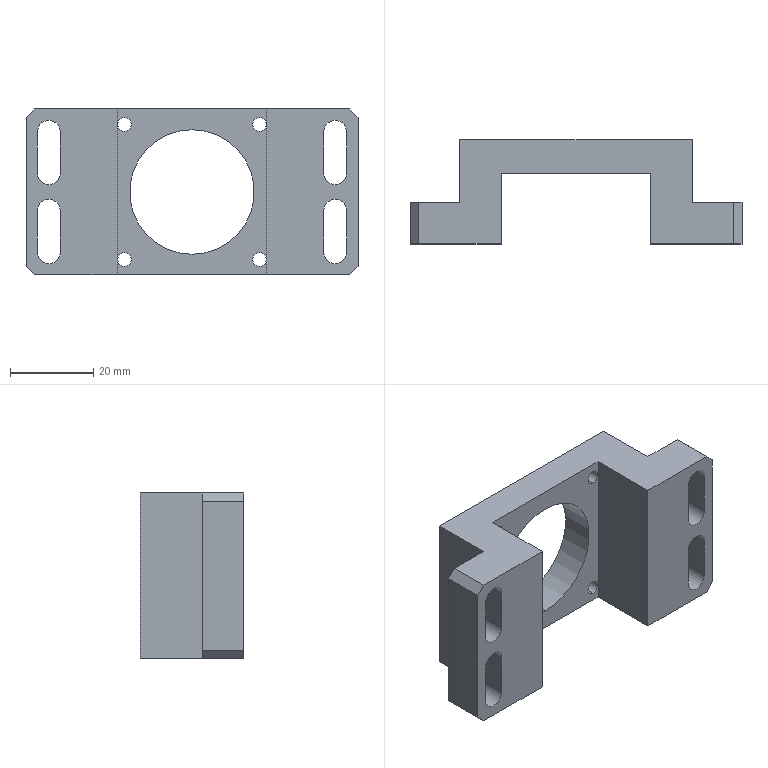Part | STEP file | 06-01-08 motor pad block | 1 solid | 48 faces | box 80 x 25 x 40 mm | volume 31958 mm3 | plane 26 | cylinder 22 | commonest cylinder face diameters 5.5 x12 3.3 x8 30.009 x2